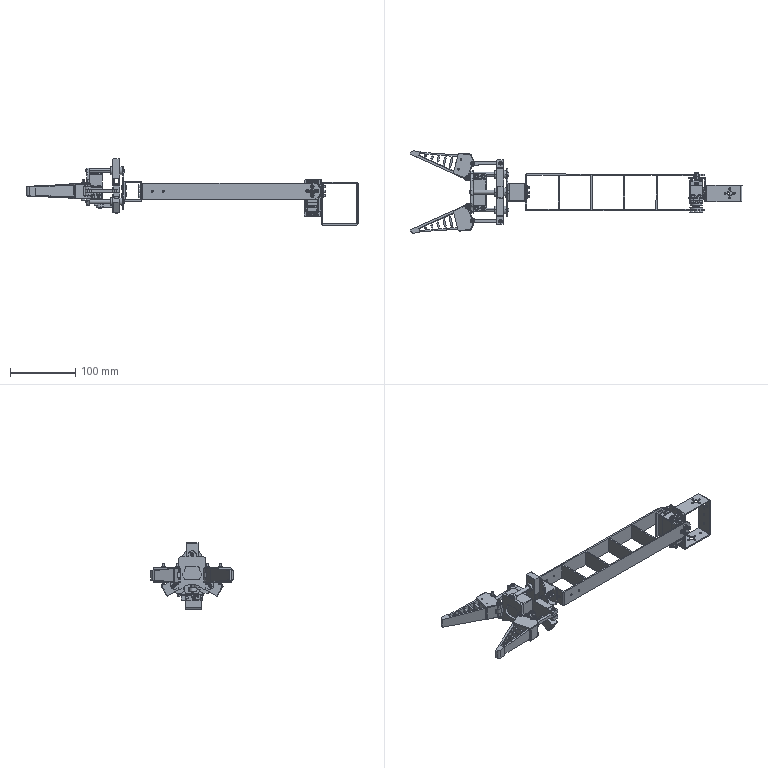Part | SolidWorks | features CompositeCurve 1 | 100 solids | 3309 faces | volume 229160 mm3 | plane 1686 | cylinder 975 | cone 422 | torus 158 | spline 38 | sphere 30 | commonest cylinder face diameters 3 x310 4 x79 6 x72 2 x54 0.4 x52 0.1 x51